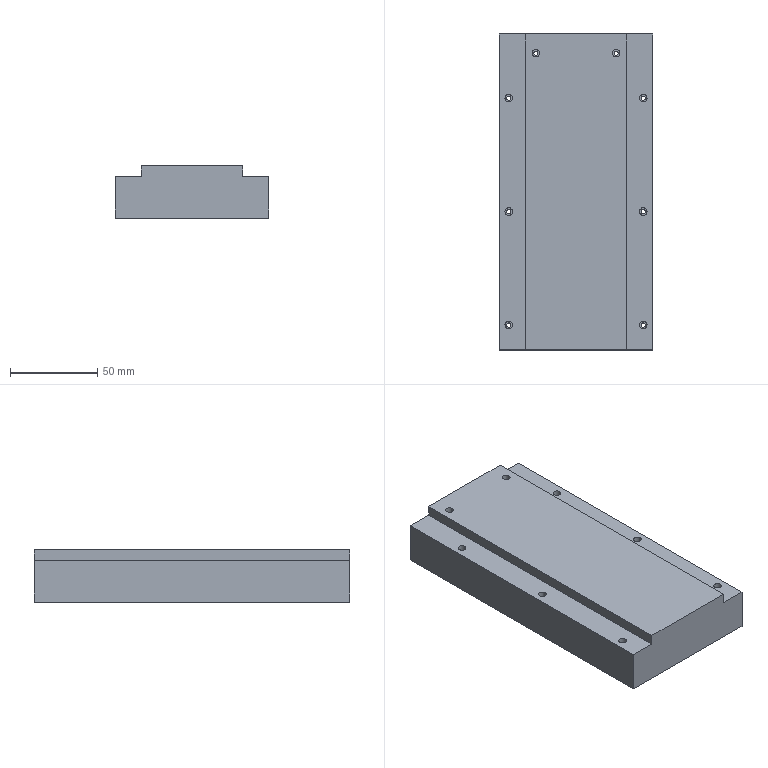NC program | NX | posted with a generic post | part box 88 x 181.05 x 30 mm
Whole program:
N10 G17 G21 G94 G90
(DYNAMIC_ROUGH_2 , TOOL : D5-15-D6-50-3T-ROUGH)
N12 T08 M6
N14 G54
N16 G17 G0 G90 X-0.04 Y-33.163 S6500 M3
N18 G43 Z52.568 H8
N20 Z3.717
N22 G94 G3 X-0.04 Y-33.163 Z3.47 I0.043 J-2.25 F3000.
N24 X-0.04 Y-33.163 Z3.223 I0.043 J-2.25
N26 X-0.04 Y-33.163 Z2.976 I0.043 J-2.25
N28 X-0.04 Y-33.163 Z2.73 I0.043 J-2.25
N30 X-0.04 Y-33.163 Z2.483 I0.043 J-2.25
N32 X-0.04 Y-33.163 Z2.236 I0.043 J-2.25
N34 X-0.04 Y-33.163 Z1.989 I0.043 J-2.25
N36 X-0.04 Y-33.163 Z1.743 I0.043 J-2.25
N38 X-0.04 Y-33.163 Z1.496 I0.043 J-2.25
N40 X-0.04 Y-33.163 Z1.249 I0.043 J-2.25
N42 X-0.04 Y-33.163 Z1.002 I0.043 J-2.25
N44 X-0.04 Y-33.163 Z0.756 I0.043 J-2.25
N46 X-0.04 Y-33.163 Z0.509 I0.043 J-2.25
N48 X-0.04 Y-33.163 Z0.262 I0.043 J-2.25
N50 X-0.04 Y-33.163 Z0.015 I0.043 J-2.25
N52 X-0.04 Y-33.163 Z-0.232 I0.043 J-2.25
N54 X-0.04 Y-33.163 Z-0.478 I0.043 J-2.25
N56 X-0.04 Y-33.163 Z-0.725 I0.043 J-2.25
N58 X-0.04 Y-33.163 Z-0.972 I0.043 J-2.25
N60 X-0.04 Y-33.163 Z-1.219 I0.043 J-2.25
N62 X-0.04 Y-33.163 Z-1.465 I0.043 J-2.25
N64 X-0.04 Y-33.163 Z-1.712 I0.043 J-2.25
N66 X-0.04 Y-33.163 Z-1.959 I0.043 J-2.25
N68 X-0.04 Y-33.163 Z-2.206 I0.043 J-2.25
N70 X-0.04 Y-33.163 Z-2.452 I0.043 J-2.25
N72 X-0.04 Y-33.163 Z-2.699 I0.043 J-2.25
N74 X-0.04 Y-33.163 Z-2.946 I0.043 J-2.25
N76 X-0.04 Y-33.163 Z-3.193 I0.043 J-2.25
N78 X-0.04 Y-33.163 Z-3.439 I0.043 J-2.25
N80 X-0.04 Y-33.163 Z-3.686 I0.043 J-2.25
N82 X-0.04 Y-33.163 Z-3.933 I0.043 J-2.25
N84 X-0.04 Y-33.163 Z-4.18 I0.043 J-2.25
N86 X-0.04 Y-33.163 Z-4.427 I0.043 J-2.25
N88 X-0.04 Y-33.163 Z-4.673 I0.043 J-2.25
N90 X-0.04 Y-33.163 Z-4.92 I0.043 J-2.25
N92 X-0.04 Y-33.163 Z-5.167 I0.043 J-2.25
N94 X-0.04 Y-33.163 Z-5.414 I0.043 J-2.25
N96 X-0.04 Y-33.163 Z-5.66 I0.043 J-2.25
N98 X-0.04 Y-33.163 Z-5.907 I0.043 J-2.25
N100 X-0.04 Y-33.163 Z-6.154 I0.043 J-2.25
N102 X-0.04 Y-33.163 Z-6.401 I0.043 J-2.25
N104 X-0.04 Y-33.163 Z-6.647 I0.043 J-2.25
N106 X-0.04 Y-33.163 Z-6.894 I0.043 J-2.25
N108 X-0.04 Y-33.163 Z-7.141 I0.043 J-2.25
N110 X-0.04 Y-33.163 Z-7.388 I0.043 J-2.25
N112 X-0.04 Y-33.163 Z-7.634 I0.043 J-2.25
N114 X-0.04 Y-33.163 Z-7.881 I0.043 J-2.25
N116 X-0.04 Y-33.163 Z-8.128 I0.043 J-2.25
N118 X-0.04 Y-33.163 Z-8.375 I0.043 J-2.25
N120 X-0.04 Y-33.163 Z-8.622 I0.043 J-2.25
N122 X-0.04 Y-33.163 Z-8.868 I0.043 J-2.25
N124 X-0.04 Y-33.163 Z-9.115 I0.043 J-2.25
N126 X-0.04 Y-33.163 Z-9.362 I0.043 J-2.25
N128 X-0.04 Y-33.163 Z-9.609 I0.043 J-2.25
N130 X-0.04 Y-33.163 Z-9.855 I0.043 J-2.25
N132 X-0.04 Y-33.163 Z-10.102 I0.043 J-2.25
N134 X-0.04 Y-33.163 Z-10.349 I0.043 J-2.25
N136 X-0.04 Y-33.163 Z-10.596 I0.043 J-2.25
N138 X2.252 Y-35.412 Z-10.78 R-2.25
N140 X-0.627 Y-37.618 R-2.272
N142 X2.278 Y-36.019 R2.406
N144 X-0.657 Y-32.999 R2.38
N146 X1.919 Y-37.092 R-2.524
N148 X-0.696 Y-32.754 R2.629
N150 X2.016 Y-37.359 R-2.772
N152 X-1.032 Y-32.588 R2.892
N154 X1.909 Y-37.806 R-3.032
N156 X-1.32 Y-32.416 R3.162
N158 X1.863 Y-38.175 R-3.302
N160 X-1.56 Y-32.219 R3.44
N162 X1.914 Y-38.478 R-3.584
N164 X-1.555 Y-31.9 R3.726
N166 X1.9 Y-38.822 R-3.872
N168 X-1.687 Y-31.634 R4.02
N170 X2.018 Y-39.101 R-4.171
N172 X-1.554 Y-31.25 R4.322
N174 X2.089 Y-39.413 R-4.477
N176 X-1.348 Y-30.854 R4.63
N178 X1.666 Y-39.939 R-4.788
N180 X-1.312 Y-30.513 R4.947
N182 X1.624 Y-40.295 R-5.109
N184 X-1.233 Y-30.158 R5.27
N186 X1.045 Y-40.782 R5.434
N188 X-0.861 Y-29.751 R5.598
N190 X0.389 Y-41.201 R5.764
N192 X5.92 Y-34.892 R5.933
N194 X-0.442 Y-29.365 R5.933
N196 X-0.323 Y-41.544 R6.102
N198 X6.274 Y-35.612 R6.273
N200 X0.285 Y-29.013 R6.273
N202 X-1.342 Y-41.755 R6.444
N204 X1.596 Y-28.858 R6.615
N206 X-2.633 Y-41.713 R6.786
N208 X3.156 Y-29.064 R6.96
N210 X-4.353 Y-41.12 R7.132
N212 X5.056 Y-29.97 R7.305
N214 X-7.23 Y-37.511 R7.472
N216 X7.55 Y-36.894 R7.624
N218 X-5.983 Y-30.291 R7.773
N220 X2.596 Y-42.942 R7.928
N222 X-0.952 Y-27.248 R8.091
N224 X-1.375 Y-43.6 R8.261
N226 X3.928 Y-27.809 R8.431
N228 X-6.32 Y-41.321 R8.601
N230 X7.798 Y-31.159 R8.771
N232 X-8.996 Y-35.997 R8.941
N234 X8.837 Y-37.919 R9.108
N236 X-7.844 Y-30.261 R9.278
N238 X6.148 Y-42.673 R9.454
N240 X-2.011 Y-25.874 R9.627
N242 X-1.631 Y-45.111 R9.794
N244 X4.796 Y-26.541 R9.96
N246 X-9.334 Y-39.471 R10.121
N248 X10.37 Y-35.714 R10.285
N250 X-10.194 Y-32.685 R10.458
N252 X9.834 Y-39.697 R10.642
N254 X-7.938 Y-27.884 R10.826
N256 X6.364 Y-44.483 R11.014
N258 X-1.743 Y-24.233 R11.197
N260 X-4.627 Y-45.831 R11.359
N262 X9.622 Y-28.897 R11.513
N264 X-11.635 Y-37.091 R11.68
N266 X11.953 Y-35.863 R11.861
N268 X-11.942 Y-33.183 R12.052
N270 X11.945 Y-38.54 R12.249
N272 X3.101 Y-23.317 R12.449
N274 X-12.114 Y-32.131 R12.449
N276 X12.088 Y-39.467 R12.651
N278 X4.037 Y-23.172 R12.852
N280 X-12.295 Y-31.334 R12.852
N282 X11.796 Y-41.223 R13.054
N284 X-12.399 Y-30.431 R-13.257
N286 X11.861 Y-41.98 R13.462
N288 X-12.41 Y-29.44 R-13.666
N290 X12.06 Y-42.462 R13.872
N292 X-12.317 Y-28.381 R-14.076
N294 X11.749 Y-43.703 R14.282
N296 X-5.754 Y-22.011 R14.482
N298 X3.527 Y-49.724 R14.665
N300 X4.19 Y-21.063 R14.844
N302 X-14.129 Y-40.587 R14.985
N304 X15.155 Y-37.187 R15.154
N306 X-14.77 Y-30.912 R15.348
N308 X14.003 Y-42.405 R15.548
N310 X-13.348 Y-26.86 R15.751
N312 X12.354 Y-45.668 R15.956
N314 X-11.206 Y-23.624 R16.159
N316 X7.364 Y-50.118 R16.359
N318 X0.641 Y-18.769 R16.551
N320 X-12.864 Y-46.16 R16.715
N322 X16.656 Y-32.123 R16.87
N324 X-17.141 Y-35.345 R17.057
N326 X15.382 Y-43.435 R17.246
N328 X17.35 Y-36.675 R17.106
N330 X17.308 Y-33.633 R36.905
N332 X-16.679 Y-29.884 R17.477
N334 X-17.349 Y-32.627 R18.319
N336 X-17.331 Y-37.924 R171.83
N338 X-14.215 Y-45.833 R16.297
N340 X17.35 Y-39.462 R17.723
N342 G1 X17.34 Y-31.838
N344 G3 X15.795 Y-27.038 R13.299
N346 X-17.349 Y-30.607 R17.922
N348 G1 Y-32.632
N350 G2 X-17.326 Y-30.1 R34.546
N352 X-15.971 Y-26.542 R11.257
N354 X16.886 Y-28.853 R18.163
N356 X17.35 Y-30.422 R14.925
N358 G1 Y-31.997
N360 G3 X17.329 Y-29.476 R44.9
N362 X15.985 Y-25.951 R10.221
N364 X-17.074 Y-27.807 R18.585
N366 X-17.349 Y-28.595 R5.835
N368 G1 Y-30.395
N370 G2 X-17.329 Y-28.248 R32.76
N372 X-16.185 Y-25.529 R8.519
N374 X16.293 Y-25.965 R18.849
N376 X17.35 Y-28.496 R10.955
N378 G1 Y-29.734
N380 G3 X17.316 Y-27.703 R18.536
N382 X15.984 Y-24.644 R8.81
N384 X-2.423 Y-16.173 R19.16
N386 X-16.82 Y-25.763 R19.138
N388 X-17.349 Y-26.977 R5.407
N390 G1 Y-28.477
N392 G2 X-17.323 Y-26.66 R17.459
N394 X-16.143 Y-24.186 R7.582
N396 X15.798 Y-23.895 R19.533
N398 X17.35 Y-26.95 R10.03
N400 G1 Y-28.037
N402 G3 X17.312 Y-26.237 R13.241
N404 X16.004 Y-23.473 R7.831
N406 X5.956 Y-16.242 R19.328
N408 X-16.271 Y-23.596 R19.948
N410 X-17.346 Y-25.55 R7.668
N412 G1 X-17.349 Y-26.9
N414 G2 X-17.32 Y-25.278 R12.303
N416 X-16.089 Y-22.929 R6.988
N418 X-2.488 Y-15.194 R19.986
N420 X15.68 Y-22.588 R20.088
N422 X17.346 Y-25.562 R9.54
N424 G1 X17.35 Y-26.574
N426 G3 X17.319 Y-24.983 R11.578
N428 X16.071 Y-22.439 R6.876
N430 X8.785 Y-16.581 R19.092
N432 X-15.909 Y-21.976 R20.666
N434 X-17.338 Y-24.238 R9.222
N436 G1 X-17.349 Y-25.475
N438 X-17.335 Y-24.106
N440 G2 X-16.284 Y-22.077 R5.593
N442 X-9.228 Y-16.435 R19.443
N444 X15.122 Y-20.865 R20.89
N446 X17.273 Y-24.088 R10.759
N448 G1 X17.35 Y-24.366
N450 Y-25.228
N452 G3 X17.305 Y-23.723 R8.635
N454 X15.967 Y-21.227 R6.778
N456 X9.118 Y-15.945 R19.214
N458 X-15.645 Y-20.61 R21.358
N460 X-17.33 Y-23.027 R9.562
N462 X-17.349 Y-24.263 R11.411
N464 G1 X-17.333 Y-22.927
N466 G2 X-16.214 Y-20.913 R5.413
N468 X-9.636 Y-15.833 R19.555
N470 X14.818 Y-19.557 R21.575
N472 X17.194 Y-22.751 R11.027
N474 X17.35 Y-23.209 R6.687
N476 G1 Y-24.034
N478 G3 X17.298 Y-22.578 R7.315
N480 X15.891 Y-20.112 R6.591
N482 X9.451 Y-15.306 R19.226
N484 X-15.46 Y-19.408 R22.037
N486 X-17.327 Y-21.908 R9.245
N488 X-17.349 Y-23.078 R9.197
N490 G1 X-17.333 Y-21.822
N492 G2 X-16.195 Y-19.861 R5.171
N494 X-10.338 Y-15.378 R19.287
N496 X-2.842 Y-13.061 R22.521
N498 X2.501 Y-13.083 R179.978
N500 X15.434 Y-19.212 R21.079
N502 X17.331 Y-22.018 R8.445
N504 X17.35 Y-22.916 R11.95
N506 G3 X17.301 Y-21.526 R6.98
N508 X15.976 Y-19.226 R6.095
N510 X10.335 Y-14.938 R18.56
N512 X5.197 Y-13.061 R21.959
N514 G1 X2.009
N516 G2 X5.846 Y-13.082 R79.502
N518 X9.79 Y-14.372 R14.015
N520 X15.936 Y-18.795 R19.184
N522 X17.347 Y-21.057 R6.456
N524 G1 X17.35 Y-21.844
N526 G3 X17.305 Y-20.528 R6.46
N528 X15.98 Y-18.272 R5.746
N530 X10.457 Y-14.193 R18.227
N532 X7.631 Y-13.061 R16.5
N534 G1 X5.568
N536 G2 X8.097 Y-13.089 R30.408
N538 X11.289 Y-14.332 R11.201
N540 X16.258 Y-18.217 R17.042
N542 X17.345 Y-20.045 R5.699
N544 G1 X17.35 Y-20.834
N546 G3 X17.303 Y-19.531 R6.549
N548 X15.949 Y-17.302 R5.623
N550 X9.527 Y-13.065 R16.717
N552 G1 X7.802 Y-13.061
N554 G2 X9.823 Y-13.082 R27.508
N556 X12.58 Y-14.266 R8.822
N558 X16.64 Y-17.766 R14.035
N560 X17.35 Y-19.117 R3.822
N562 G1 Y-19.829
N564 G3 X17.296 Y-18.545 R5.712
N566 X15.859 Y-16.291 R5.661
N568 X11.138 Y-13.072 R13.864
N570 G1 X9.639 Y-13.061
N572 G2 X11.382 Y-13.088 R15.813
N574 X13.915 Y-14.319 R7.621
N576 X16.99 Y-17.363 R10.589
N578 X17.35 Y-18.177 R2.631
N580 G1 Y-18.89
N582 G3 X17.296 Y-17.612 R5.633
N584 X15.887 Y-15.432 R5.407
N586 X12.501 Y-13.07 R10.191
N588 G1 X11.157 Y-13.061
N590 G2 X12.732 Y-13.09 R12.213
N592 X15.162 Y-14.443 R6.546
N594 X17.269 Y-16.986 R7.258
N596 G1 X17.35 Y-17.252
N598 Y-17.927
N600 G3 X17.297 Y-16.71 R5.368
N602 X15.847 Y-14.544 R5.116
N604 X13.723 Y-13.074 R7.2
N606 G1 X12.515 Y-13.061
N608 X13.854 Y-13.078
N610 G2 X15.965 Y-14.354 R4.947
N612 X17.345 Y-16.321 R4.943
N614 G1 X17.35 Y-17.039
N616 G3 X17.294 Y-15.826 R5.045
N618 X15.579 Y-13.568 R4.701
N620 X14.661 Y-13.061 R2.279
N622 G1 X13.686
N624 G2 X14.873 Y-13.081 R18.547
N626 X16.92 Y-14.664 R3.984
N628 X17.35 Y-15.539 R2.336
N630 G1 Y-16.176
N632 G3 X17.288 Y-14.997 R4.409
N634 X15.616 Y-13.083 R3.464
N636 X14.714 Y-13.061 R6.601
N638 G2 X15.677 Y-13.079 R35.599
N640 X17.345 Y-14.745 R2.722
N642 G1 X17.35 Y-15.349
N644 G3 X17.282 Y-14.287 R3.389
N646 X16.229 Y-13.08 R2.066
N648 G1 X15.555 Y-13.061
N650 G2 X16.328 Y-13.087 R3.614
N652 X17.35 Y-14.199 R1.626
N654 G1 Y-14.612
N656 G3 X17.271 Y-13.741 R2.204
N658 X16.579 Y-13.065 R1.037
N660 G1 X16.167 Y-13.061
N662 G2 X16.845 Y-13.133 R1.393
N664 X17.35 Y-14.064 R0.897
N666 G3 X17.198 Y-13.284 R1.15
N668 X16.594 Y-13.061 R0.625
N670 G2 X17.324 Y-13.428 R0.657
N672 G1 X17.35 Y-13.667
N674 G3 X17.249 Y-13.28 R0.631
N676 X16.983 Y-13.087 R0.615
N678 X16.39 Y-13.414 R0.511
N680 G1 X15.993 Y-14.23 Z-10.688
N682 X15.946 Y-14.288 Z-10.68
N684 G2 X15.578 Y-14.449 R0.506 F15000.
N686 G1 X-1.474 Y-14.429
N688 G2 X-1.81 Y-14.299 R0.509
N690 G1 X-1.917 Y-14.162 Z-10.698 F3000.
N692 X-2.004 Y-14.011 Z-10.715
N694 X-2.321 Y-13.463 Z-10.78
N696 X-2.408 Y-13.312
N698 X-2.521 Y-13.178
N700 G3 X-2.842 Y-13.061 R0.51
N702 X-5.2 Y-13.13 R16.41
N704 X-11.509 Y-15.501 R18.934
N706 X-16.482 Y-19.544 R18.292
N708 X-17.343 Y-20.917 R4.617
N710 G1 X-17.35 Y-21.982
N712 G2 X-17.33 Y-20.753 R16.537
N714 X-16.192 Y-18.866 R4.976
N716 X-10.677 Y-14.741 R18.944
N718 X-6.177 Y-13.061 R19.219
N720 G1 X-4.527
N722 G3 X-7.263 Y-13.089 R35.799
N724 X-10.998 Y-14.411 R12.435
N726 X-16.395 Y-18.455 R18.338
N728 X-17.342 Y-19.891 R4.701
N730 G1 X-17.35 Y-20.927
N732 G2 X-17.331 Y-19.74 R21.08
N734 X-16.165 Y-17.871 R4.802
N736 X-8.367 Y-13.075 R18.167
N738 G1 X-6.931 Y-13.061
N740 G3 X-9.145 Y-13.092 R22.942
N742 X-12.485 Y-14.43 R10.343
N744 X-16.685 Y-17.841 R15.335
N746 X-17.341 Y-18.898 R3.756
N748 G1 X-17.35 Y-19.906
N750 G2 X-17.33 Y-18.753 R14.608
N752 X-16.238 Y-17.011 R4.477
N754 X-10.123 Y-13.086 R15.149
N756 X-8.833 Y-13.061 R9.207
N758 G3 X-10.715 Y-13.087 R18.774
N760 X-13.618 Y-14.324 R8.453
N762 X-16.994 Y-17.31 R11.8
N764 X-17.35 Y-18.002 R1.786
N766 G1 Y-18.902
N768 G2 X-17.327 Y-17.786 R8.404
N770 X-16.164 Y-16.02 R4.506
N772 X-11.56 Y-13.07 R11.789
N774 G1 X-10.474 Y-13.061
N776 G3 X-12.203 Y-13.101 R11.992
N778 X-15.158 Y-14.585 R7.793
N780 X-17.305 Y-16.9 R7.504
N782 G1 X-17.35 Y-17.081
N784 Y-17.944
N786 G2 X-17.328 Y-16.867 R8.559
N788 X-16.152 Y-15.139 R4.252
N790 X-12.864 Y-13.066 R8.631
N792 G1 X-11.885 Y-13.061
N794 G3 X-13.48 Y-13.106 R9.604
N796 X-17.308 Y-16.021 R6.521
N798 G1 X-17.35 Y-16.203
N800 Y-17.028
N802 G2 X-17.329 Y-15.989 R8.402
N804 X-16.119 Y-14.314 R3.879
N806 X-14.021 Y-13.065 R5.875
N808 G1 X-13.159 Y-13.061
N810 G3 X-14.6 Y-13.112 R7.3
N812 X-17.319 Y-15.235 R4.629
N814 X-17.35 Y-16.132 R4.245
N816 G2 X-17.324 Y-15.165 R4.714
N818 X-15.829 Y-13.451 R3.506
N820 X-14.979 Y-13.061 R2.681
N822 G1 X-14.267
N824 G3 X-15.472 Y-13.1 R6.338
N826 X-17.33 Y-14.57 R2.93
N828 X-17.35 Y-15.318 R8.587
N830 G2 X-17.324 Y-14.471 R3.966
N832 X-15.772 Y-13.061 R2.365
N834 G1 X-15.21
N836 G3 X-16.272 Y-13.128 R3.457
N838 X-17.331 Y-14.03 R1.746
N840 G1 X-17.35 Y-14.628
N842 G2 X-17.32 Y-13.926 R2.527
N844 X-16.335 Y-13.061 R1.423
N846 G1 X-15.923
N848 G3 X-16.803 Y-13.15 R2.032
N850 X-17.35 Y-14.074 R0.823
N852 G2 X-17.216 Y-13.389 R0.97
N854 X-16.465 Y-13.061 R0.764
N856 G3 X-17.193 Y-13.231 R0.944
N858 X-17.35 Y-13.743 R0.662
N860 G2 X-16.872 Y-13.07 R0.566
N862 X-16.341 Y-13.351 R0.501
N864 G1 X-16.03 Y-14.283 Z-10.68
N866 X-15.911 Y-14.664 F15000.
N868 X-15.905 Y-14.744
N870 X-15.981 Y-36.284
N872 G2 X-16.112 Y-36.62 R0.509
N874 G1 X-16.248 Y-36.727 Z-10.698 F3000.
N876 X-16.399 Y-36.813 Z-10.715
N878 X-16.948 Y-37.131 Z-10.78
N880 X-17.099 Y-37.219
N882 X-17.232 Y-37.331
N884 G3 X-17.349 Y-37.652 R0.51
N886 X-17.306 Y-39.91 R20.455
N888 X-15.414 Y-44.816 R13.645
N890 X17.346 Y-41.082 R18.151
N892 G1 X17.35 Y-39.432
N894 G2 X17.318 Y-41.49 R19.854
N896 X15.999 Y-44.681 R10.53
N898 X-16.474 Y-43.382 R18.38
N900 X-17.348 Y-40.926 R13.122
N902 G1 X-17.349 Y-39.426
N904 G3 X-17.326 Y-41.802 R36.328
N906 X-16.029 Y-45.131 R9.655
N908 X10.968 Y-50.81 R18.777
N910 X17.26 Y-43.107 R17.962
N912 G1 X17.35 Y-42.807
N914 Y-41.157
N916 G2 X17.328 Y-43.122 R22.956
N918 X16.14 Y-45.781 R8.156
N920 X-16.062 Y-45.586 R19.061
N922 X-17.348 Y-42.73 R10.834
N924 G1 Y-41.53
N926 G3 X-17.323 Y-43.446 R20.539
N928 X-16.101 Y-46.299 R8.123
N930 X-3.64 Y-54.62 R19.104
N932 X16.606 Y-45.856 R19.46
N934 X17.346 Y-44.345 R7.825
N936 G1 X17.35 Y-42.883
N938 G2 X17.321 Y-44.628 R14.165
N940 X16.096 Y-47.078 R7.44
N942 X-7.615 Y-53.687 R19.735
N944 X-16.42 Y-46.272 R18.948
N946 X-17.348 Y-44.224 R8.032
N948 G1 Y-43.211
N950 G3 X-17.319 Y-44.873 R13.12
N952 X-16.044 Y-47.576 R7.417
N954 X-7.244 Y-54.32 R19.23
N956 X16.191 Y-47.699 R20.174
N958 X17.34 Y-45.718 R9.1
N960 G1 X17.35 Y-44.406
N962 G2 X17.32 Y-45.948 R11.043
N964 X16.097 Y-48.227 R6.752
N966 X4.161 Y-55.549 R20.049
N968 X-15.447 Y-48.798 R20.333
N970 X-17.34 Y-45.608 R10.098
N972 G1 X-17.348 Y-44.605
N974 G3 X-17.308 Y-46.183 R10.624
N976 X-15.973 Y-48.789 R7.044
N978 X-8.375 Y-54.627 R19.339
N980 X15.735 Y-49.38 R20.903
N982 X17.333 Y-46.977 R9.733
N984 G1 X17.35 Y-45.749
N986 X17.335 Y-47.086
N988 G2 X16.289 Y-49.07 R5.44
N990 X9.528 Y-54.465 R19.368
N992 X-14.927 Y-50.417 R21.12
N994 X-17.257 Y-47.061 R10.96
N996 G1 X-17.348 Y-46.751
N998 Y-45.851
N1000 G3 X-17.31 Y-47.343 R9.277
N1002 X-16.016 Y-49.79 R6.438
N1004 X-9.608 Y-54.842 R18.977
N1006 X15.521 Y-50.652 R21.591
N1008 X17.333 Y-48.128 R9.314
N1010 G1 X17.35 Y-46.935
N1012 X17.335 Y-48.232
N1014 G2 X16.235 Y-50.195 R5.245
N1016 X10.069 Y-54.999 R19.305
N1018 X-14.56 Y-51.754 R21.817
N1020 X-17.138 Y-48.463 R11.562
N1022 X-17.348 Y-47.878 R3.153
N1024 G1 Y-47.016
N1026 G3 X-17.3 Y-48.494 R7.994
N1028 X-15.911 Y-50.934 R6.405
N1030 X-9.741 Y-55.579 R19.056
N1032 X-1.935 Y-57.761 R22.377
N1034 X2.153 Y-57.733 R77.591
N1036 X15.673 Y-51.489 R21.694
N1038 X17.329 Y-49.233 R8.51
N1040 X17.35 Y-48.071 R8.423
N1042 G2 X17.332 Y-49.328 R54.185
N1044 X16.223 Y-51.226 R5.041
N1046 X10.572 Y-55.553 R19.031
N1048 X4.053 Y-57.761 R22.366
N1050 G1 X1.69
N1052 G3 X5.531 Y-57.742 R107.348
N1054 X9.9 Y-56.384 R14.745
N1056 X16.19 Y-51.915 R19.832
N1058 X17.335 Y-50.256 R6.466
N1060 G1 X17.35 Y-49.186
N1062 G2 X17.332 Y-50.369 R37.501
N1064 X16.214 Y-52.22 R4.809
N1066 X10.746 Y-56.272 R18.709
N1068 X6.811 Y-57.761 R17.683
N1070 G1 X5.274
N1072 G3 X7.833 Y-57.731 R29.424
N1074 X11.525 Y-56.359 R11.996
N1076 X16.441 Y-52.599 R17.62
N1078 X17.337 Y-51.254 R5.195
N1080 G1 X17.35 Y-50.233
N1082 G2 X17.329 Y-51.387 R11.056
N1084 X16.169 Y-53.225 R4.752
N1086 X8.892 Y-57.743 R17.386
N1088 X7.506 Y-57.761 R20.679
N1090 G3 X9.587 Y-57.735 R22.229
N1092 X12.695 Y-56.495 R9.538
N1094 X16.761 Y-53.162 R14.461
N1096 X17.347 Y-52.173 R2.845
N1098 G1 X17.35 Y-51.238
N1100 X17.332 Y-52.345
N1102 G2 X16.183 Y-54.141 R4.508
N1104 X10.55 Y-57.742 R14.296
N1106 X9.315 Y-57.761 R12.461
N1108 G3 X11.173 Y-57.728 R15.937
N1110 X14.071 Y-56.435 R8.373
N1112 X17.082 Y-53.654 R10.579
N1114 X17.35 Y-53.09 R1.43
N1116 G1 Y-52.19
N1118 G2 X17.33 Y-53.298 R14.888
N1120 X16.194 Y-55.029 R4.329
N1122 X11.948 Y-57.753 R10.883
N1124 G1 X10.87 Y-57.761
N1126 G3 X12.561 Y-57.724 R12.459
N1128 X15.41 Y-56.273 R7.266
N1130 X17.317 Y-54.157 R6.734
N1132 X17.35 Y-53.145 R4.661
N1134 G2 X17.329 Y-54.215 R11.101
N1136 X16.133 Y-55.941 R4.193
N1138 X13.213 Y-57.756 R7.797
N1140 G1 X12.233 Y-57.761
N1142 G3 X13.756 Y-57.728 R10.017
N1144 X17.311 Y-55.038 R5.877
N1146 X17.35 Y-54.081 R3.718
N1148 G2 X17.327 Y-55.082 R6.904
N1150 X16.062 Y-56.765 R3.813
N1152 X14.318 Y-57.759 R5.108
N1154 G1 X13.499 Y-57.761
N1156 G3 X14.815 Y-57.727 R7.771
N1158 X17.32 Y-55.801 R4.13
N1160 X17.35 Y-54.942 R4.297
N1162 G2 X17.327 Y-55.863 R6.004
N1164 X15.732 Y-57.566 R3.256
N1166 X15.233 Y-57.761 R2.147
N1168 G1 X14.558
N1170 G3 X15.772 Y-57.702 R4.742
N1172 X17.321 Y-56.457 R2.731
N1174 X17.35 Y-55.71 R3.205
N1176 G2 X17.322 Y-56.525 R3.395
N1178 X15.951 Y-57.761 R2.032
N1180 G1 X15.426
N1182 G3 X16.376 Y-57.713 R3.393
N1184 X17.333 Y-56.905 R1.483
N1186 G1 X17.35 Y-56.351
N1188 G2 X17.32 Y-57.014 R2.462
N1190 X16.464 Y-57.761 R1.22
N1192 G1 X16.127
N1194 G3 X16.987 Y-57.627 R1.492
N1196 X17.35 Y-56.854 R0.727
N1198 G2 X17.215 Y-57.5 R0.88
N1200 X16.58 Y-57.761 R0.664
N1202 G3 X17.249 Y-57.542 R0.721
N1204 X17.35 Y-57.155 R0.676
N1206 X17.038 Y-56.692 R0.501
N1208 G1 X16.126 Y-56.327 Z-10.68
N1210 X15.937 Y-56.249 F15000.
N1212 X15.74 Y-56.191
N1214 X-0.567 Y-56.394
N1216 G3 X-0.899 Y-56.526 R0.509
N1218 G1 X-1.019 Y-56.682 Z-10.7 F3000.
N1220 X-1.116 Y-56.853 Z-10.72
N1222 X-1.413 Y-57.36 Z-10.78
N1224 X-1.502 Y-57.512
N1226 X-1.615 Y-57.645
N1228 G2 X-1.935 Y-57.761 R0.511
N1230 X-6.793 Y-57.048 R13.248
N1232 X-15.522 Y-51.758 R20.792
N1234 X-17.326 Y-49.079 R8.256
N1236 X-17.348 Y-48.175 R6.081
N1238 G3 X-17.301 Y-49.538 R7.296
N1240 X-15.987 Y-51.824 R5.937
N1242 X-10.283 Y-56.116 R18.532
N1244 X-5.901 Y-57.761 R21.046
N1246 G1 X-3.201
N1248 G2 X-6.504 Y-57.735 R52.547
N1250 X-10.196 Y-56.456 R13.276
N1252 X-16.023 Y-52.167 R18.693
N1254 X-17.345 Y-50.013 R6.12
N1256 G1 X-17.348 Y-49.196
N1258 G3 X-17.301 Y-50.553 R7.061
N1260 X-15.942 Y-52.829 R5.771
N1262 X-10.086 Y-57.007 R18.364
N1264 X-8.135 Y-57.761 R12.867
N1266 G1 X-6.185
N1268 G2 X-8.516 Y-57.742 R41.568
N1270 X-11.533 Y-56.559 R10.097
N1272 X-16.344 Y-52.736 R16.427
N1274 X-17.343 Y-51.024 R5.486
N1276 G1 X-17.348 Y-50.232
N1278 G3 X-17.297 Y-51.548 R6.284
N1280 X-15.938 Y-53.763 R5.627
N1282 X-9.974 Y-57.752 R16.281
N1284 G1 X-8.291 Y-57.761
N1286 G2 X-10.249 Y-57.737 R21.916
N1288 X-12.96 Y-56.526 R8.618
N1290 X-16.702 Y-53.203 R13.243
N1292 X-17.348 Y-51.948 R3.714
N1294 G1 Y-51.235
N1296 G3 X-17.296 Y-52.509 R5.743
N1298 X-15.877 Y-54.736 R5.57
N1300 X-11.509 Y-57.749 R13.062
N1302 G1 X-10.042 Y-57.761
N1304 G2 X-11.751 Y-57.731 R13.392
N1306 X-14.287 Y-56.444 R7.478
N1308 X-17.076 Y-53.54 R9.639
N1310 X-17.348 Y-52.883 R2.442
N1312 G1 Y-52.208
N1314 G3 X-17.292 Y-53.449 R5.258
N1316 X-15.878 Y-55.616 R5.389
N1318 X-12.817 Y-57.753 R9.238
N1320 G1 X-11.517 Y-57.761
N1322 X-12.963 Y-57.749
N1324 G2 X-15.088 Y-56.634 R5.471
N1326 X-17.274 Y-54.046 R7.092
N1328 G1 X-17.348 Y-53.792
N1330 Y-53.117
N1332 G3 X-17.293 Y-54.338 R5.324
N1334 X-15.799 Y-56.523 R5.055
N1336 X-13.995 Y-57.748 R6.357
N1338 G1 X-12.863 Y-57.761
N1340 G2 X-14.13 Y-57.742 R25.32
N1342 X-16.219 Y-56.411 R4.733
N1344 X-17.344 Y-54.707 R4.372
N1346 G1 X-17.348 Y-53.995
N1348 G3 X-17.289 Y-55.215 R4.916
N1350 X-14.977 Y-57.747 R4.468
N1352 G1 X-13.987 Y-57.761
N1354 G2 X-15.095 Y-57.741 R14.477
N1356 X-17.341 Y-55.541 R3.698
N1358 G1 X-17.348 Y-54.886
N1360 G3 X-17.285 Y-56.018 R4.054
N1362 X-15.787 Y-57.74 R3.11
N1364 X-14.961 Y-57.761 R6.628
N1366 G2 X-15.882 Y-57.737 R5.072
N1368 X-17.342 Y-56.24 R2.486
N1370 G1 X-17.348 Y-55.674
N1372 G3 X-17.276 Y-56.695 R3.051
N1374 X-16.364 Y-57.739 R1.846
N1376 X-15.724 Y-57.761 R5.81
N1378 G2 X-16.457 Y-57.733 R2.9
N1380 X-17.348 Y-56.739 R1.425
N1382 G1 Y-56.364
N1384 G3 X-17.224 Y-57.274 R1.745
N1386 X-16.625 Y-57.761 R0.818
N1388 G1 X-16.288
N1390 G2 X-16.927 Y-57.684 R1.205
N1392 X-17.348 Y-56.877 R0.792
N1394 G3 X-17.177 Y-57.601 R0.935
N1396 X-16.629 Y-57.761 R0.685
N1398 G2 X-17.339 Y-57.283 R0.588
N1400 X-16.986 Y-56.72 R0.505
N1402 G1 X-16.12 Y-56.459
N1404 X-16.096 Y-56.452 Z-10.779
N1406 X-16.072 Y-56.445 Z-10.777
N1408 X-16.048 Y-56.438 Z-10.774
N1410 X-16.024 Y-56.431 Z-10.77
N1412 X-16. Y-56.423 Z-10.764
N1414 X-15.976 Y-56.416 Z-10.757
N1416 X-15.952 Y-56.409 Z-10.748
N1418 X-15.928 Y-56.402 Z-10.738
N1420 X-15.904 Y-56.395 Z-10.726
N1422 X-15.88 Y-56.387 Z-10.713
N1424 X-15.856 Y-56.38 Z-10.698
N1426 X-15.832 Y-56.373 Z-10.68
N1428 X-15.808 Y-56.366 Z-10.66
N1430 X-15.785 Y-56.359 Z-10.637
N1432 X-15.761 Y-56.351 Z-10.611
N1434 X-15.737 Y-56.344 Z-10.58
N1436 X-15.713 Y-56.337 Z-10.543
N1438 X-15.689 Y-56.33 Z-10.498
N1440 X-15.665 Y-56.322 Z-10.436
N1442 X-15.641 Y-56.315 Z-10.28
N1444 G0 Z52.568
N1446 M5
(LOW_WALL_ROUGH_FACE , TOOL : D6-18-D6-50-3T-FINISH)
N1448 T09 M6
N1450 G54
N1452 G17 G0 G90 X0.7 Y-32.671 S4500 M3
N1454 G43 Z52.518 H9
N1456 Z-8.88
N1458 G94 G1 Y-29.711 Z-9.139 F600.
N1460 X-0.7 Z-9.261
N1462 Y-41.111 Z-10.259
N1464 X0.7 Z-10.381
N1466 Y-35.411 Z-10.88
N1468 Y-29.711
N1470 X-0.7
N1472 Y-41.111
N1474 X0.7
N1476 Y-35.411
N1478 X3.4
N1480 Y-27.011
N1482 X-3.4
N1484 Y-43.811
N1486 X3.4
N1488 Y-35.411
N1490 X7.9
N1492 Y-22.511
N1494 X-7.9
N1496 Y-48.311
N1498 X7.9
N1500 Y-35.411
N1502 X12.4
N1504 Y-18.011
N1506 X-12.4
N1508 Y-52.811
N1510 X12.4
N1512 Y-35.411
N1514 X16.9
N1516 Y-13.511
N1518 X-16.9
N1520 Y-57.311
N1522 X16.9
N1524 Y-35.411
N1526 Y-34.411
N1528 Z-9.88
N1530 G0 Z52.518
(LOW_WALL_ROUGH_FACE_COPY , TOOL : D6-18-D6-50-3T-FINISH)
N1532 X-15. Y-15.411
N1534 Z52.418
N1536 Z-8.88
N1538 G1 Z-10.88
N1540 X-15.999 Y-14.412
N1542 G3 X-16.999 Y-13.412 R1.
N1544 G1 Y-57.41
N1546 X16.999
N1548 Y-13.412
N1550 X-16.999
N1552 X-17. Y-14.412
N1554 G3 X-16. Y-15.412 R1.
N1556 G1 X-15.
N1558 Z-8.88
N1560 G0 Z52.418
N1562 M5
N1564 M2